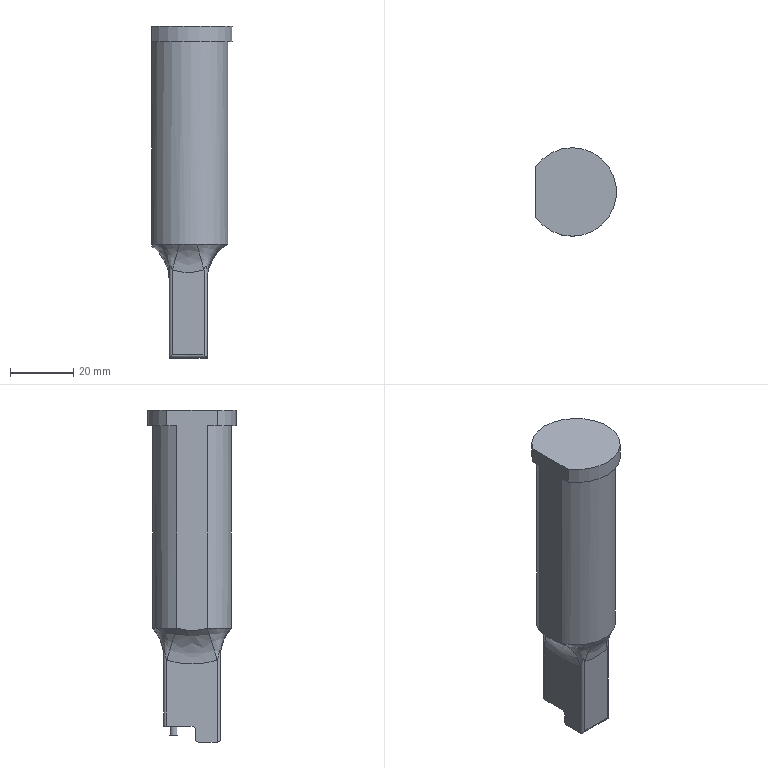Part | STEP file | lll_id3170_x_t | 1 solid | 29 faces | box 25.5 x 28 x 105 mm | volume 41911 mm3 | plane 11 | cylinder 10 | spline 8 | commonest cylinder face diameters 2 x7 2.4 x1 25 x1 28 x1
STEP:
#1=CARTESIAN_POINT('',(481.37,-342.601,87.5));
#2=VERTEX_POINT('',#1);
#3=CARTESIAN_POINT('',(481.37,-352.399,87.5));
#4=VERTEX_POINT('',#3);
#5=CARTESIAN_POINT('',(492.87,-347.5,87.5));
#6=DIRECTION('',(0.,0.,-1.));
#7=DIRECTION('',(-1.,0.,0.));
#8=AXIS2_PLACEMENT_3D('',#5,#6,#7);
#9=CIRCLE('',#8,12.5);
#10=EDGE_CURVE('',#2,#4,#9,.T.);
#11=ORIENTED_EDGE('',*,*,#10,.T.);
#12=CARTESIAN_POINT('',(481.37,-352.399,23.5));
#13=VERTEX_POINT('',#12);
#14=CARTESIAN_POINT('',(481.37,-352.399,-7.5));
#15=DIRECTION('',(0.,0.,1.));
#16=VECTOR('',#15,1.);
#17=LINE('',#14,#16);
#18=EDGE_CURVE('',#13,#4,#17,.T.);
#19=ORIENTED_EDGE('',*,*,#18,.F.);
#20=CARTESIAN_POINT('',(490.1,-359.689,23.5));
#21=VERTEX_POINT('',#20);
#22=CARTESIAN_POINT('',(490.1,-359.689,23.5));
#23=CARTESIAN_POINT('',(486.235,-358.811,23.5));
#24=CARTESIAN_POINT('',(482.924,-356.046,23.499));
#25=CARTESIAN_POINT('',(481.37,-352.399,23.5));
#26=B_SPLINE_CURVE_WITH_KNOTS('',3,(#22,#23,#24,#25),.UNSPECIFIED.,.F.,.F.,(4,4),(0.,1.),.UNSPECIFIED.);
#27=EDGE_CURVE('',#21,#13,#26,.T.);
#28=ORIENTED_EDGE('',*,*,#27,.F.);
#29=CARTESIAN_POINT('',(495.641,-359.689,23.5));
#30=VERTEX_POINT('',#29);
#31=CARTESIAN_POINT('',(495.641,-359.689,23.5));
#32=CARTESIAN_POINT('',(493.82,-360.103,23.5));
#33=CARTESIAN_POINT('',(491.921,-360.103,23.5));
#34=CARTESIAN_POINT('',(490.1,-359.689,23.5));
#35=B_SPLINE_CURVE_WITH_KNOTS('',3,(#31,#32,#33,#34),.UNSPECIFIED.,.F.,.F.,(4,4),(0.,1.),.UNSPECIFIED.);
#36=EDGE_CURVE('',#30,#21,#35,.T.);
#37=ORIENTED_EDGE('',*,*,#36,.F.);
#38=CARTESIAN_POINT('',(504.391,-352.351,23.5));
#39=VERTEX_POINT('',#38);
#40=CARTESIAN_POINT('',(504.391,-352.351,23.5));
#41=CARTESIAN_POINT('',(502.846,-356.02,23.5));
#42=CARTESIAN_POINT('',(499.523,-358.807,23.5));
#43=CARTESIAN_POINT('',(495.641,-359.689,23.5));
#44=B_SPLINE_CURVE_WITH_KNOTS('',3,(#40,#41,#42,#43),.UNSPECIFIED.,.F.,.F.,(4,4),(0.,1.),.UNSPECIFIED.);
#45=EDGE_CURVE('',#39,#30,#44,.T.);
#46=ORIENTED_EDGE('',*,*,#45,.F.);
#47=CARTESIAN_POINT('',(504.391,-342.649,23.5));
#48=VERTEX_POINT('',#47);
#49=CARTESIAN_POINT('',(504.391,-342.649,23.5));
#50=CARTESIAN_POINT('',(505.688,-345.731,23.5));
#51=CARTESIAN_POINT('',(505.688,-349.27,23.5));
#52=CARTESIAN_POINT('',(504.391,-352.351,23.5));
#53=B_SPLINE_CURVE_WITH_KNOTS('',3,(#49,#50,#51,#52),.UNSPECIFIED.,.F.,.F.,(4,4),(0.,1.),.UNSPECIFIED.);
#54=EDGE_CURVE('',#48,#39,#53,.T.);
#55=ORIENTED_EDGE('',*,*,#54,.F.);
#56=CARTESIAN_POINT('',(495.641,-335.311,23.5));
#57=VERTEX_POINT('',#56);
#58=CARTESIAN_POINT('',(495.641,-335.311,23.5));
#59=CARTESIAN_POINT('',(499.523,-336.193,23.5));
#60=CARTESIAN_POINT('',(502.846,-338.98,23.5));
#61=CARTESIAN_POINT('',(504.391,-342.649,23.5));
#62=B_SPLINE_CURVE_WITH_KNOTS('',3,(#58,#59,#60,#61),.UNSPECIFIED.,.F.,.F.,(4,4),(0.,1.),.UNSPECIFIED.);
#63=EDGE_CURVE('',#57,#48,#62,.T.);
#64=ORIENTED_EDGE('',*,*,#63,.F.);
#65=CARTESIAN_POINT('',(490.1,-335.311,23.5));
#66=VERTEX_POINT('',#65);
#67=CARTESIAN_POINT('',(490.1,-335.311,23.5));
#68=CARTESIAN_POINT('',(491.921,-334.897,23.5));
#69=CARTESIAN_POINT('',(493.82,-334.897,23.5));
#70=CARTESIAN_POINT('',(495.641,-335.311,23.5));
#71=B_SPLINE_CURVE_WITH_KNOTS('',3,(#67,#68,#69,#70),.UNSPECIFIED.,.F.,.F.,(4,4),(0.,1.),.UNSPECIFIED.);
#72=EDGE_CURVE('',#66,#57,#71,.T.);
#73=ORIENTED_EDGE('',*,*,#72,.F.);
#74=CARTESIAN_POINT('',(481.37,-342.601,23.5));
#75=VERTEX_POINT('',#74);
#76=CARTESIAN_POINT('',(481.37,-342.601,23.5));
#77=CARTESIAN_POINT('',(482.924,-338.955,23.5));
#78=CARTESIAN_POINT('',(486.235,-336.189,23.5));
#79=CARTESIAN_POINT('',(490.1,-335.311,23.5));
#80=B_SPLINE_CURVE_WITH_KNOTS('',3,(#76,#77,#78,#79),.UNSPECIFIED.,.F.,.F.,(4,4),(0.,1.),.UNSPECIFIED.);
#81=EDGE_CURVE('',#75,#66,#80,.T.);
#82=ORIENTED_EDGE('',*,*,#81,.F.);
#83=CARTESIAN_POINT('',(481.37,-342.601,-7.5));
#84=DIRECTION('',(0.,0.,-1.));
#85=VECTOR('',#84,1.);
#86=LINE('',#83,#85);
#87=EDGE_CURVE('',#2,#75,#86,.T.);
#88=ORIENTED_EDGE('',*,*,#87,.F.);
#89=EDGE_LOOP('',(#11,#19,#28,#37,#46,#55,#64,#73,#82,#88));
#90=FACE_OUTER_BOUND('',#89,.T.);
#91=CARTESIAN_POINT('',(492.87,-347.5,-7.5));
#92=DIRECTION('',(0.,0.,1.));
#93=DIRECTION('',(-1.,0.,0.));
#94=AXIS2_PLACEMENT_3D('',#91,#92,#93);
#95=CYLINDRICAL_SURFACE('',#94,12.5);
#96=ADVANCED_FACE('',(#90),#95,.T.);
#97=CARTESIAN_POINT('',(481.37,-355.484,87.5));
#98=VERTEX_POINT('',#97);
#99=CARTESIAN_POINT('',(481.37,-347.5,87.5));
#100=DIRECTION('',(0.,-1.,0.));
#101=VECTOR('',#100,1.);
#102=LINE('',#99,#101);
#103=EDGE_CURVE('',#4,#98,#102,.T.);
#104=ORIENTED_EDGE('',*,*,#103,.F.);
#105=ORIENTED_EDGE('',*,*,#10,.F.);
#106=CARTESIAN_POINT('',(481.37,-339.516,87.5));
#107=VERTEX_POINT('',#106);
#108=CARTESIAN_POINT('',(481.37,-347.5,87.5));
#109=DIRECTION('',(0.,-1.,0.));
#110=VECTOR('',#109,1.);
#111=LINE('',#108,#110);
#112=EDGE_CURVE('',#107,#2,#111,.T.);
#113=ORIENTED_EDGE('',*,*,#112,.F.);
#114=CARTESIAN_POINT('',(492.87,-347.5,87.5));
#115=DIRECTION('',(0.,0.,1.));
#116=DIRECTION('',(-1.,0.,0.));
#117=AXIS2_PLACEMENT_3D('',#114,#115,#116);
#118=CIRCLE('',#117,14.);
#119=EDGE_CURVE('',#98,#107,#118,.T.);
#120=ORIENTED_EDGE('',*,*,#119,.F.);
#121=EDGE_LOOP('',(#104,#105,#113,#120));
#122=FACE_OUTER_BOUND('',#121,.T.);
#123=CARTESIAN_POINT('',(492.87,-347.5,87.5));
#124=DIRECTION('',(0.,0.,1.));
#125=DIRECTION('',(-1.,0.,0.));
#126=AXIS2_PLACEMENT_3D('',#123,#124,#125);
#127=PLANE('',#126);
#128=ADVANCED_FACE('',(#122),#127,.F.);
#129=CARTESIAN_POINT('',(481.37,-355.484,92.5));
#130=VERTEX_POINT('',#129);
#131=CARTESIAN_POINT('',(481.37,-339.516,92.5));
#132=VERTEX_POINT('',#131);
#133=CARTESIAN_POINT('',(492.87,-347.5,92.5));
#134=DIRECTION('',(0.,0.,1.));
#135=DIRECTION('',(1.,0.,0.));
#136=AXIS2_PLACEMENT_3D('',#133,#134,#135);
#137=CIRCLE('',#136,14.);
#138=EDGE_CURVE('',#130,#132,#137,.T.);
#139=ORIENTED_EDGE('',*,*,#138,.T.);
#140=CARTESIAN_POINT('',(481.37,-21.,92.5));
#141=DIRECTION('',(0.,1.,0.));
#142=VECTOR('',#141,1.);
#143=LINE('',#140,#142);
#144=EDGE_CURVE('',#130,#132,#143,.T.);
#145=ORIENTED_EDGE('',*,*,#144,.F.);
#146=EDGE_LOOP('',(#139,#145));
#147=FACE_OUTER_BOUND('',#146,.T.);
#148=CARTESIAN_POINT('',(444.,-21.,92.5));
#149=DIRECTION('',(0.,0.,-1.));
#150=DIRECTION('',(1.,0.,0.));
#151=AXIS2_PLACEMENT_3D('',#148,#149,#150);
#152=PLANE('',#151);
#153=ADVANCED_FACE('',(#147),#152,.F.);
#154=ORIENTED_EDGE('',*,*,#138,.F.);
#155=CARTESIAN_POINT('',(481.37,-355.484,-7.5));
#156=DIRECTION('',(0.,0.,1.));
#157=VECTOR('',#156,1.);
#158=LINE('',#155,#157);
#159=EDGE_CURVE('',#98,#130,#158,.T.);
#160=ORIENTED_EDGE('',*,*,#159,.F.);
#161=ORIENTED_EDGE('',*,*,#119,.T.);
#162=CARTESIAN_POINT('',(481.37,-339.516,-7.5));
#163=DIRECTION('',(0.,0.,-1.));
#164=VECTOR('',#163,1.);
#165=LINE('',#162,#164);
#166=EDGE_CURVE('',#132,#107,#165,.T.);
#167=ORIENTED_EDGE('',*,*,#166,.F.);
#168=EDGE_LOOP('',(#154,#160,#161,#167));
#169=FACE_OUTER_BOUND('',#168,.T.);
#170=CARTESIAN_POINT('',(492.87,-347.5,-7.5));
#171=DIRECTION('',(0.,0.,1.));
#172=DIRECTION('',(-1.,0.,0.));
#173=AXIS2_PLACEMENT_3D('',#170,#171,#172);
#174=CYLINDRICAL_SURFACE('',#173,14.);
#175=ADVANCED_FACE('',(#169),#174,.T.);
#176=CARTESIAN_POINT('',(481.37,-352.355,23.486));
#177=VERTEX_POINT('',#176);
#178=CARTESIAN_POINT('',(481.37,-352.399,23.5));
#179=CARTESIAN_POINT('',(481.37,-352.384,23.495));
#180=CARTESIAN_POINT('',(481.37,-352.37,23.491));
#181=CARTESIAN_POINT('',(481.37,-352.355,23.486));
#182=B_SPLINE_CURVE_WITH_KNOTS('',3,(#178,#179,#180,#181),.UNSPECIFIED.,.F.,.F.,(4,4),(0.,1.),.UNSPECIFIED.);
#183=EDGE_CURVE('',#13,#177,#182,.T.);
#184=ORIENTED_EDGE('',*,*,#183,.T.);
#185=CARTESIAN_POINT('',(486.87,-355.5,13.344));
#186=VERTEX_POINT('',#185);
#187=CARTESIAN_POINT('',(473.87,-355.5,13.344));
#188=DIRECTION('',(0.,0.9551,-0.2962));
#189=DIRECTION('',(0.,-0.2962,-0.9551));
#190=AXIS2_PLACEMENT_3D('',#187,#188,#189);
#191=CIRCLE('',#190,13.);
#192=EDGE_CURVE('',#177,#186,#191,.T.);
#193=ORIENTED_EDGE('',*,*,#192,.T.);
#194=CARTESIAN_POINT('',(487.87,-356.5,15.267));
#195=VERTEX_POINT('',#194);
#196=CARTESIAN_POINT('',(486.87,-355.5,13.344));
#197=CARTESIAN_POINT('',(486.87,-355.629,13.906));
#198=CARTESIAN_POINT('',(486.895,-355.755,14.475));
#199=CARTESIAN_POINT('',(486.992,-355.995,15.517));
#200=CARTESIAN_POINT('',(487.065,-356.107,15.974));
#201=CARTESIAN_POINT('',(487.251,-356.296,16.492));
#202=CARTESIAN_POINT('',(487.365,-356.373,16.537));
#203=CARTESIAN_POINT('',(487.61,-356.475,16.162));
#204=CARTESIAN_POINT('',(487.743,-356.5,15.752));
#205=CARTESIAN_POINT('',(487.87,-356.5,15.267));
#206=(BOUNDED_CURVE()B_SPLINE_CURVE(3,(#196,#197,#198,#199,#200,#201,#202,#203,#204,#205),.UNSPECIFIED.,.F.,.F.)B_SPLINE_CURVE_WITH_KNOTS((4,2,2,2,4),(0.,0.25,0.5,0.75,1.),.UNSPECIFIED.)CURVE()GEOMETRIC_REPRESENTATION_ITEM()RATIONAL_B_SPLINE_CURVE((1.,1.,1.,1.,1.,1.,1.,1.,1.,1.))REPRESENTATION_ITEM(''));
#207=EDGE_CURVE('',#186,#195,#206,.T.);
#208=ORIENTED_EDGE('',*,*,#207,.T.);
#209=CARTESIAN_POINT('',(487.87,-369.5,15.267));
#210=DIRECTION('',(0.9652,0.,-0.2614));
#211=DIRECTION('',(0.2614,0.,0.9652));
#212=AXIS2_PLACEMENT_3D('',#209,#210,#211);
#213=CIRCLE('',#212,13.);
#214=EDGE_CURVE('',#195,#21,#213,.T.);
#215=ORIENTED_EDGE('',*,*,#214,.T.);
#216=ORIENTED_EDGE('',*,*,#27,.T.);
#217=EDGE_LOOP('',(#184,#193,#208,#215,#216));
#218=FACE_OUTER_BOUND('',#217,.T.);
#219=CARTESIAN_POINT('',(486.87,-355.5,13.344));
#220=CARTESIAN_POINT('',(486.87,-353.501,19.791));
#221=CARTESIAN_POINT('',(481.35,-352.351,23.5));
#222=CARTESIAN_POINT('',(486.87,-355.629,13.906));
#223=CARTESIAN_POINT('',(486.616,-353.761,19.745));
#224=CARTESIAN_POINT('',(481.743,-353.285,23.5));
#225=CARTESIAN_POINT('',(486.895,-355.755,14.475));
#226=CARTESIAN_POINT('',(486.443,-354.143,19.805));
#227=CARTESIAN_POINT('',(482.223,-354.123,23.5));
#228=CARTESIAN_POINT('',(486.992,-355.995,15.517));
#229=CARTESIAN_POINT('',(486.389,-354.985,20.001));
#230=CARTESIAN_POINT('',(483.391,-355.708,23.5));
#231=CARTESIAN_POINT('',(487.065,-356.107,15.974));
#232=CARTESIAN_POINT('',(486.509,-355.437,20.135));
#233=CARTESIAN_POINT('',(484.07,-356.432,23.5));
#234=CARTESIAN_POINT('',(487.251,-356.296,16.492));
#235=CARTESIAN_POINT('',(487.023,-356.169,20.292));
#236=CARTESIAN_POINT('',(485.587,-357.707,23.5));
#237=CARTESIAN_POINT('',(487.365,-356.373,16.537));
#238=CARTESIAN_POINT('',(487.422,-356.453,20.308));
#239=CARTESIAN_POINT('',(486.438,-358.263,23.5));
#240=CARTESIAN_POINT('',(487.61,-356.475,16.162));
#241=CARTESIAN_POINT('',(488.285,-356.698,20.191));
#242=CARTESIAN_POINT('',(488.213,-359.142,23.5));
#243=CARTESIAN_POINT('',(487.743,-356.5,15.752));
#244=CARTESIAN_POINT('',(488.759,-356.66,20.063));
#245=CARTESIAN_POINT('',(489.162,-359.476,23.5));
#246=CARTESIAN_POINT('',(487.87,-356.5,15.267));
#247=CARTESIAN_POINT('',(489.141,-356.5,19.959));
#248=CARTESIAN_POINT('',(490.1,-359.689,23.5));
#249=(BOUNDED_SURFACE()B_SPLINE_SURFACE(3,2,((#219,#220,#221),(#222,#223,#224),(#225,#226,#227),(#228,#229,#230),(#231,#232,#233),(#234,#235,#236),(#237,#238,#239),(#240,#241,#242),(#243,#244,#245),(#246,#247,#248)),.UNSPECIFIED.,.F.,.F.,.F.)B_SPLINE_SURFACE_WITH_KNOTS((4,2,2,2,4),(3,3),(0.,0.25,0.5,0.75,1.),(0.,1.),.UNSPECIFIED.)GEOMETRIC_REPRESENTATION_ITEM()RATIONAL_B_SPLINE_SURFACE(((1.,0.8875,1.),(1.,0.9048,1.),(1.,0.9192,1.),(1.,0.9424,1.),(1.,0.9508,1.),(1.,0.96,1.),(1.,0.9607,1.),(1.,0.9542,1.),(1.,0.9469,1.),(1.,0.9367,1.)))REPRESENTATION_ITEM('')SURFACE());
#250=ADVANCED_FACE('',(#218),#249,.T.);
#251=CARTESIAN_POINT('',(481.37,-342.645,23.486));
#252=VERTEX_POINT('',#251);
#253=CARTESIAN_POINT('',(481.37,-352.355,23.486));
#254=CARTESIAN_POINT('',(481.37,-350.783,22.999));
#255=CARTESIAN_POINT('',(481.37,-349.135,22.86));
#256=CARTESIAN_POINT('',(481.37,-345.863,22.86));
#257=CARTESIAN_POINT('',(481.37,-344.22,22.998));
#258=CARTESIAN_POINT('',(481.37,-342.645,23.486));
#259=B_SPLINE_CURVE_WITH_KNOTS('',3,(#253,#254,#255,#256,#257,#258),.UNSPECIFIED.,.F.,.F.,(4,2,4),(0.,0.5,1.),.UNSPECIFIED.);
#260=EDGE_CURVE('',#177,#252,#259,.T.);
#261=ORIENTED_EDGE('',*,*,#260,.T.);
#262=CARTESIAN_POINT('',(486.87,-339.5,13.344));
#263=VERTEX_POINT('',#262);
#264=CARTESIAN_POINT('',(473.87,-339.5,13.344));
#265=DIRECTION('',(0.,0.9551,0.2962));
#266=DIRECTION('',(0.,0.2962,-0.9551));
#267=AXIS2_PLACEMENT_3D('',#264,#265,#266);
#268=CIRCLE('',#267,13.);
#269=EDGE_CURVE('',#252,#263,#268,.T.);
#270=ORIENTED_EDGE('',*,*,#269,.T.);
#271=CARTESIAN_POINT('',(486.87,-339.5,13.344));
#272=CARTESIAN_POINT('',(486.87,-342.08,12.544));
#273=CARTESIAN_POINT('',(486.87,-344.771,12.243));
#274=CARTESIAN_POINT('',(486.87,-350.203,12.241));
#275=CARTESIAN_POINT('',(486.87,-352.893,12.536));
#276=CARTESIAN_POINT('',(486.87,-355.5,13.344));
#277=B_SPLINE_CURVE_WITH_KNOTS('',3,(#271,#272,#273,#274,#275,#276),.UNSPECIFIED.,.F.,.F.,(4,2,4),(0.,0.5,1.),.UNSPECIFIED.);
#278=EDGE_CURVE('',#263,#186,#277,.T.);
#279=ORIENTED_EDGE('',*,*,#278,.T.);
#280=ORIENTED_EDGE('',*,*,#192,.F.);
#281=EDGE_LOOP('',(#261,#270,#279,#280));
#282=FACE_OUTER_BOUND('',#281,.T.);
#283=CARTESIAN_POINT('',(486.87,-339.5,13.344));
#284=CARTESIAN_POINT('',(486.87,-341.499,19.791));
#285=CARTESIAN_POINT('',(481.35,-342.649,23.5));
#286=CARTESIAN_POINT('',(486.87,-342.068,12.548));
#287=CARTESIAN_POINT('',(486.87,-343.348,19.674));
#288=CARTESIAN_POINT('',(480.798,-343.961,23.5));
#289=CARTESIAN_POINT('',(486.87,-344.771,12.243));
#290=CARTESIAN_POINT('',(486.87,-345.394,19.747));
#291=CARTESIAN_POINT('',(480.372,-345.705,23.5));
#292=CARTESIAN_POINT('',(486.87,-350.203,12.241));
#293=CARTESIAN_POINT('',(486.87,-349.586,19.747));
#294=CARTESIAN_POINT('',(480.369,-349.278,23.5));
#295=CARTESIAN_POINT('',(486.87,-352.886,12.534));
#296=CARTESIAN_POINT('',(486.87,-351.616,19.672));
#297=CARTESIAN_POINT('',(480.787,-351.013,23.5));
#298=CARTESIAN_POINT('',(486.87,-355.5,13.344));
#299=CARTESIAN_POINT('',(486.87,-353.501,19.791));
#300=CARTESIAN_POINT('',(481.35,-352.351,23.5));
#301=(BOUNDED_SURFACE()B_SPLINE_SURFACE(3,2,((#283,#284,#285),(#286,#287,#288),(#289,#290,#291),(#292,#293,#294),(#295,#296,#297),(#298,#299,#300)),.UNSPECIFIED.,.F.,.F.,.F.)B_SPLINE_SURFACE_WITH_KNOTS((4,2,4),(3,3),(0.,0.5,1.),(0.,1.),.UNSPECIFIED.)GEOMETRIC_REPRESENTATION_ITEM()RATIONAL_B_SPLINE_SURFACE(((1.,0.8875,1.),(1.,0.8752,1.),(1.,0.8661,1.),(1.,0.866,1.),(1.,0.875,1.),(1.,0.8875,1.)))REPRESENTATION_ITEM('')SURFACE());
#302=ADVANCED_FACE('',(#282),#301,.T.);
#303=CARTESIAN_POINT('',(481.37,-342.601,23.5));
#304=CARTESIAN_POINT('',(481.37,-342.616,23.495));
#305=CARTESIAN_POINT('',(481.37,-342.63,23.491));
#306=CARTESIAN_POINT('',(481.37,-342.645,23.486));
#307=B_SPLINE_CURVE_WITH_KNOTS('',3,(#303,#304,#305,#306),.UNSPECIFIED.,.F.,.F.,(4,4),(0.,1.),.UNSPECIFIED.);
#308=EDGE_CURVE('',#75,#252,#307,.T.);
#309=ORIENTED_EDGE('',*,*,#308,.F.);
#310=ORIENTED_EDGE('',*,*,#81,.T.);
#311=CARTESIAN_POINT('',(487.87,-338.5,15.267));
#312=VERTEX_POINT('',#311);
#313=CARTESIAN_POINT('',(487.87,-325.5,15.267));
#314=DIRECTION('',(0.9652,0.,-0.2614));
#315=DIRECTION('',(-0.2614,0.,-0.9652));
#316=AXIS2_PLACEMENT_3D('',#313,#314,#315);
#317=CIRCLE('',#316,13.);
#318=EDGE_CURVE('',#66,#312,#317,.T.);
#319=ORIENTED_EDGE('',*,*,#318,.T.);
#320=CARTESIAN_POINT('',(487.87,-338.5,15.267));
#321=CARTESIAN_POINT('',(487.741,-338.5,15.757));
#322=CARTESIAN_POINT('',(487.609,-338.526,16.165));
#323=CARTESIAN_POINT('',(487.425,-338.602,16.444));
#324=CARTESIAN_POINT('',(487.365,-338.635,16.484));
#325=CARTESIAN_POINT('',(487.254,-338.71,16.441));
#326=CARTESIAN_POINT('',(487.203,-338.752,16.361));
#327=CARTESIAN_POINT('',(487.064,-338.894,15.97));
#328=CARTESIAN_POINT('',(486.992,-339.005,15.517));
#329=CARTESIAN_POINT('',(486.895,-339.246,14.474));
#330=CARTESIAN_POINT('',(486.87,-339.372,13.9));
#331=CARTESIAN_POINT('',(486.87,-339.5,13.344));
#332=(BOUNDED_CURVE()B_SPLINE_CURVE(3,(#320,#321,#322,#323,#324,#325,#326,#327,#328,#329,#330,#331),.UNSPECIFIED.,.F.,.F.)B_SPLINE_CURVE_WITH_KNOTS((4,2,2,2,2,4),(0.,0.25,0.375,0.5,0.75,1.),.UNSPECIFIED.)CURVE()GEOMETRIC_REPRESENTATION_ITEM()RATIONAL_B_SPLINE_CURVE((1.,1.,1.,1.,1.,1.,1.,1.,1.,1.,1.,1.))REPRESENTATION_ITEM(''));
#333=EDGE_CURVE('',#312,#263,#332,.T.);
#334=ORIENTED_EDGE('',*,*,#333,.T.);
#335=ORIENTED_EDGE('',*,*,#269,.F.);
#336=EDGE_LOOP('',(#309,#310,#319,#334,#335));
#337=FACE_OUTER_BOUND('',#336,.T.);
#338=CARTESIAN_POINT('',(487.87,-338.5,15.267));
#339=CARTESIAN_POINT('',(489.141,-338.5,19.959));
#340=CARTESIAN_POINT('',(490.1,-335.311,23.5));
#341=CARTESIAN_POINT('',(487.741,-338.5,15.757));
#342=CARTESIAN_POINT('',(488.754,-338.338,20.065));
#343=CARTESIAN_POINT('',(489.151,-335.527,23.5));
#344=CARTESIAN_POINT('',(487.609,-338.526,16.165));
#345=CARTESIAN_POINT('',(488.281,-338.303,20.192));
#346=CARTESIAN_POINT('',(488.206,-335.86,23.5));
#347=CARTESIAN_POINT('',(487.425,-338.602,16.444));
#348=CARTESIAN_POINT('',(487.632,-338.488,20.28));
#349=CARTESIAN_POINT('',(486.872,-336.522,23.5));
#350=CARTESIAN_POINT('',(487.365,-338.635,16.484));
#351=CARTESIAN_POINT('',(487.421,-338.589,20.293));
#352=CARTESIAN_POINT('',(486.432,-336.774,23.5));
#353=CARTESIAN_POINT('',(487.254,-338.71,16.441));
#354=CARTESIAN_POINT('',(487.052,-338.853,20.279));
#355=CARTESIAN_POINT('',(485.597,-337.322,23.5));
#356=CARTESIAN_POINT('',(487.203,-338.752,16.361));
#357=CARTESIAN_POINT('',(486.893,-339.015,20.253));
#358=CARTESIAN_POINT('',(485.201,-337.617,23.5));
#359=CARTESIAN_POINT('',(487.064,-338.894,15.97));
#360=CARTESIAN_POINT('',(486.507,-339.567,20.133));
#361=CARTESIAN_POINT('',(484.062,-338.575,23.5));
#362=CARTESIAN_POINT('',(486.992,-339.005,15.517));
#363=CARTESIAN_POINT('',(486.389,-340.015,20.001));
#364=CARTESIAN_POINT('',(483.391,-339.292,23.5));
#365=CARTESIAN_POINT('',(486.895,-339.246,14.474));
#366=CARTESIAN_POINT('',(486.443,-340.858,19.804));
#367=CARTESIAN_POINT('',(482.223,-340.879,23.5));
#368=CARTESIAN_POINT('',(486.87,-339.372,13.9));
#369=CARTESIAN_POINT('',(486.618,-341.241,19.745));
#370=CARTESIAN_POINT('',(481.74,-341.724,23.5));
#371=CARTESIAN_POINT('',(486.87,-339.5,13.344));
#372=CARTESIAN_POINT('',(486.87,-341.499,19.791));
#373=CARTESIAN_POINT('',(481.35,-342.649,23.5));
#374=(BOUNDED_SURFACE()B_SPLINE_SURFACE(3,2,((#338,#339,#340),(#341,#342,#343),(#344,#345,#346),(#347,#348,#349),(#350,#351,#352),(#353,#354,#355),(#356,#357,#358),(#359,#360,#361),(#362,#363,#364),(#365,#366,#367),(#368,#369,#370),(#371,#372,#373)),.UNSPECIFIED.,.F.,.F.,.F.)B_SPLINE_SURFACE_WITH_KNOTS((4,2,2,2,2,4),(3,3),(0.,0.25,0.375,0.5,0.75,1.),(0.,1.),.UNSPECIFIED.)GEOMETRIC_REPRESENTATION_ITEM()RATIONAL_B_SPLINE_SURFACE(((1.,0.9367,1.),(1.,0.947,1.),(1.,0.9542,1.),(1.,0.9591,1.),(1.,0.9597,1.),(1.,0.959,1.),(1.,0.9576,1.),(1.,0.9507,1.),(1.,0.9424,1.),(1.,0.9192,1.),(1.,0.9047,1.),(1.,0.8875,1.)))REPRESENTATION_ITEM('')SURFACE());
#375=ADVANCED_FACE('',(#337),#374,.T.);
#376=CARTESIAN_POINT('',(491.67,-341.7,-7.5));
#377=VERTEX_POINT('',#376);
#378=CARTESIAN_POINT('',(492.87,-341.7,-7.5));
#379=DIRECTION('',(0.,0.,1.));
#380=DIRECTION('',(-1.,0.,0.));
#381=AXIS2_PLACEMENT_3D('',#378,#379,#380);
#382=CIRCLE('',#381,1.2);
#383=EDGE_CURVE('',#377,#377,#382,.T.);
#384=ORIENTED_EDGE('',*,*,#383,.T.);
#385=EDGE_LOOP('',(#384));
#386=FACE_BOUND('',#385,.T.);
#387=CARTESIAN_POINT('',(486.87,-339.5,-7.5));
#388=VERTEX_POINT('',#387);
#389=CARTESIAN_POINT('',(486.87,-347.5,-7.5));
#390=VERTEX_POINT('',#389);
#391=CARTESIAN_POINT('',(486.87,-339.5,-7.5));
#392=DIRECTION('',(0.,-1.,0.));
#393=VECTOR('',#392,1.);
#394=LINE('',#391,#393);
#395=EDGE_CURVE('',#388,#390,#394,.T.);
#396=ORIENTED_EDGE('',*,*,#395,.F.);
#397=CARTESIAN_POINT('',(487.87,-338.5,-7.5));
#398=VERTEX_POINT('',#397);
#399=CARTESIAN_POINT('',(487.87,-339.5,-7.5));
#400=DIRECTION('',(0.,0.,1.));
#401=DIRECTION('',(-1.,0.,0.));
#402=AXIS2_PLACEMENT_3D('',#399,#400,#401);
#403=CIRCLE('',#402,1.);
#404=EDGE_CURVE('',#398,#388,#403,.T.);
#405=ORIENTED_EDGE('',*,*,#404,.F.);
#406=CARTESIAN_POINT('',(497.87,-338.5,-7.5));
#407=VERTEX_POINT('',#406);
#408=CARTESIAN_POINT('',(497.87,-338.5,-7.5));
#409=DIRECTION('',(-1.,0.,0.));
#410=VECTOR('',#409,1.);
#411=LINE('',#408,#410);
#412=EDGE_CURVE('',#407,#398,#411,.T.);
#413=ORIENTED_EDGE('',*,*,#412,.F.);
#414=CARTESIAN_POINT('',(498.87,-339.5,-7.5));
#415=VERTEX_POINT('',#414);
#416=CARTESIAN_POINT('',(497.87,-339.5,-7.5));
#417=DIRECTION('',(0.,0.,1.));
#418=DIRECTION('',(-1.,0.,0.));
#419=AXIS2_PLACEMENT_3D('',#416,#417,#418);
#420=CIRCLE('',#419,1.);
#421=EDGE_CURVE('',#415,#407,#420,.T.);
#422=ORIENTED_EDGE('',*,*,#421,.F.);
#423=CARTESIAN_POINT('',(498.87,-347.5,-7.5));
#424=VERTEX_POINT('',#423);
#425=CARTESIAN_POINT('',(498.87,-355.5,-7.5));
#426=DIRECTION('',(0.,1.,0.));
#427=VECTOR('',#426,1.);
#428=LINE('',#425,#427);
#429=EDGE_CURVE('',#424,#415,#428,.T.);
#430=ORIENTED_EDGE('',*,*,#429,.F.);
#431=CARTESIAN_POINT('',(497.87,-347.5,-7.5));
#432=DIRECTION('',(1.,0.,0.));
#433=VECTOR('',#432,1.);
#434=LINE('',#431,#433);
#435=EDGE_CURVE('',#390,#424,#434,.T.);
#436=ORIENTED_EDGE('',*,*,#435,.F.);
#437=EDGE_LOOP('',(#396,#405,#413,#422,#430,#436));
#438=FACE_BOUND('',#437,.T.);
#439=CARTESIAN_POINT('',(497.87,-339.5,-7.5));
#440=DIRECTION('',(0.,0.,-1.));
#441=DIRECTION('',(-1.,0.,0.));
#442=AXIS2_PLACEMENT_3D('',#439,#440,#441);
#443=PLANE('',#442);
#444=ADVANCED_FACE('',(#386,#438),#443,.T.);
#445=CARTESIAN_POINT('',(497.87,-356.5,-11.5));
#446=VERTEX_POINT('',#445);
#447=CARTESIAN_POINT('',(497.87,-356.5,15.267));
#448=VERTEX_POINT('',#447);
#449=CARTESIAN_POINT('',(497.87,-356.5,-7.5));
#450=DIRECTION('',(0.,0.,1.));
#451=VECTOR('',#450,1.);
#452=LINE('',#449,#451);
#453=EDGE_CURVE('',#446,#448,#452,.T.);
#454=ORIENTED_EDGE('',*,*,#453,.T.);
#455=CARTESIAN_POINT('',(487.87,-356.5,15.267));
#456=CARTESIAN_POINT('',(489.495,-356.5,14.827));
#457=CARTESIAN_POINT('',(491.197,-356.5,14.626));
#458=CARTESIAN_POINT('',(494.549,-356.5,14.626));
#459=CARTESIAN_POINT('',(496.228,-356.5,14.823));
#460=CARTESIAN_POINT('',(497.87,-356.5,15.267));
#461=B_SPLINE_CURVE_WITH_KNOTS('',3,(#455,#456,#457,#458,#459,#460),.UNSPECIFIED.,.F.,.F.,(4,2,4),(0.,0.5,1.),.UNSPECIFIED.);
#462=EDGE_CURVE('',#195,#448,#461,.T.);
#463=ORIENTED_EDGE('',*,*,#462,.F.);
#464=CARTESIAN_POINT('',(487.87,-356.5,-11.5));
#465=VERTEX_POINT('',#464);
#466=CARTESIAN_POINT('',(487.87,-356.5,-7.5));
#467=DIRECTION('',(0.,0.,1.));
#468=VECTOR('',#467,1.);
#469=LINE('',#466,#468);
#470=EDGE_CURVE('',#465,#195,#469,.T.);
#471=ORIENTED_EDGE('',*,*,#470,.F.);
#472=CARTESIAN_POINT('',(487.87,-356.5,-11.5));
#473=DIRECTION('',(-1.,0.,0.));
#474=VECTOR('',#473,1.);
#475=LINE('',#472,#474);
#476=EDGE_CURVE('',#446,#465,#475,.T.);
#477=ORIENTED_EDGE('',*,*,#476,.F.);
#478=EDGE_LOOP('',(#454,#463,#471,#477));
#479=FACE_OUTER_BOUND('',#478,.T.);
#480=CARTESIAN_POINT('',(487.87,-356.5,-7.5));
#481=DIRECTION('',(0.,-1.,0.));
#482=DIRECTION('',(1.,0.,0.));
#483=AXIS2_PLACEMENT_3D('',#480,#481,#482);
#484=PLANE('',#483);
#485=ADVANCED_FACE('',(#479),#484,.T.);
#486=ORIENTED_EDGE('',*,*,#470,.T.);
#487=ORIENTED_EDGE('',*,*,#207,.F.);
#488=CARTESIAN_POINT('',(486.87,-355.5,-12.5));
#489=VERTEX_POINT('',#488);
#490=CARTESIAN_POINT('',(486.87,-355.5,-7.5));
#491=DIRECTION('',(0.,0.,1.));
#492=VECTOR('',#491,1.);
#493=LINE('',#490,#492);
#494=EDGE_CURVE('',#489,#186,#493,.T.);
#495=ORIENTED_EDGE('',*,*,#494,.F.);
#496=CARTESIAN_POINT('',(487.87,-355.5,-11.5));
#497=DIRECTION('',(0.7071,0.,-0.7071));
#498=DIRECTION('',(-0.7071,0.,-0.7071));
#499=AXIS2_PLACEMENT_3D('',#496,#497,#498);
#500=ELLIPSE('',#499,1.414,1.);
#501=EDGE_CURVE('',#465,#489,#500,.T.);
#502=ORIENTED_EDGE('',*,*,#501,.F.);
#503=EDGE_LOOP('',(#486,#487,#495,#502));
#504=FACE_OUTER_BOUND('',#503,.T.);
#505=CARTESIAN_POINT('',(487.87,-355.5,-7.5));
#506=DIRECTION('',(0.,0.,-1.));
#507=DIRECTION('',(1.,0.,0.));
#508=AXIS2_PLACEMENT_3D('',#505,#506,#507);
#509=CYLINDRICAL_SURFACE('',#508,1.);
#510=ADVANCED_FACE('',(#504),#509,.T.);
#511=CARTESIAN_POINT('',(486.87,-349.5,-12.5));
#512=VERTEX_POINT('',#511);
#513=CARTESIAN_POINT('',(486.87,-339.5,-12.5));
#514=DIRECTION('',(0.,-1.,0.));
#515=VECTOR('',#514,1.);
#516=LINE('',#513,#515);
#517=EDGE_CURVE('',#512,#489,#516,.T.);
#518=ORIENTED_EDGE('',*,*,#517,.T.);
#519=ORIENTED_EDGE('',*,*,#494,.T.);
#520=ORIENTED_EDGE('',*,*,#278,.F.);
#521=CARTESIAN_POINT('',(486.87,-339.5,-7.5));
#522=DIRECTION('',(0.,0.,1.));
#523=VECTOR('',#522,1.);
#524=LINE('',#521,#523);
#525=EDGE_CURVE('',#388,#263,#524,.T.);
#526=ORIENTED_EDGE('',*,*,#525,.F.);
#527=ORIENTED_EDGE('',*,*,#395,.T.);
#528=CARTESIAN_POINT('',(486.87,-348.5,-8.5));
#529=VERTEX_POINT('',#528);
#530=CARTESIAN_POINT('',(486.87,-347.5,-8.5));
#531=DIRECTION('',(-1.,0.,0.));
#532=DIRECTION('',(0.,0.,-1.));
#533=AXIS2_PLACEMENT_3D('',#530,#531,#532);
#534=CIRCLE('',#533,1.);
#535=EDGE_CURVE('',#529,#390,#534,.T.);
#536=ORIENTED_EDGE('',*,*,#535,.F.);
#537=CARTESIAN_POINT('',(486.87,-348.5,-11.5));
#538=VERTEX_POINT('',#537);
#539=CARTESIAN_POINT('',(486.87,-348.5,-7.5));
#540=DIRECTION('',(0.,0.,1.));
#541=VECTOR('',#540,1.);
#542=LINE('',#539,#541);
#543=EDGE_CURVE('',#538,#529,#542,.T.);
#544=ORIENTED_EDGE('',*,*,#543,.F.);
#545=CARTESIAN_POINT('',(486.87,-349.5,-11.5));
#546=DIRECTION('',(1.,0.,0.));
#547=DIRECTION('',(0.,0.,-1.));
#548=AXIS2_PLACEMENT_3D('',#545,#546,#547);
#549=CIRCLE('',#548,1.);
#550=EDGE_CURVE('',#512,#538,#549,.T.);
#551=ORIENTED_EDGE('',*,*,#550,.F.);
#552=EDGE_LOOP('',(#518,#519,#520,#526,#527,#536,#544,#551));
#553=FACE_OUTER_BOUND('',#552,.T.);
#554=CARTESIAN_POINT('',(486.87,-339.5,-7.5));
#555=DIRECTION('',(-1.,0.,0.));
#556=DIRECTION('',(0.,-1.,0.));
#557=AXIS2_PLACEMENT_3D('',#554,#555,#556);
#558=PLANE('',#557);
#559=ADVANCED_FACE('',(#553),#558,.T.);
#560=CARTESIAN_POINT('',(487.87,-338.5,-7.5));
#561=DIRECTION('',(0.,0.,1.));
#562=VECTOR('',#561,1.);
#563=LINE('',#560,#562);
#564=EDGE_CURVE('',#398,#312,#563,.T.);
#565=ORIENTED_EDGE('',*,*,#564,.F.);
#566=ORIENTED_EDGE('',*,*,#404,.T.);
#567=ORIENTED_EDGE('',*,*,#525,.T.);
#568=ORIENTED_EDGE('',*,*,#333,.F.);
#569=EDGE_LOOP('',(#565,#566,#567,#568));
#570=FACE_OUTER_BOUND('',#569,.T.);
#571=CARTESIAN_POINT('',(487.87,-339.5,-7.5));
#572=DIRECTION('',(0.,0.,-1.));
#573=DIRECTION('',(1.,0.,0.));
#574=AXIS2_PLACEMENT_3D('',#571,#572,#573);
#575=CYLINDRICAL_SURFACE('',#574,1.);
#576=ADVANCED_FACE('',(#570),#575,.T.);
#577=CARTESIAN_POINT('',(497.87,-338.5,15.267));
#578=VERTEX_POINT('',#577);
#579=CARTESIAN_POINT('',(497.87,-338.5,-7.5));
#580=DIRECTION('',(0.,0.,1.));
#581=VECTOR('',#580,1.);
#582=LINE('',#579,#581);
#583=EDGE_CURVE('',#407,#578,#582,.T.);
#584=ORIENTED_EDGE('',*,*,#583,.F.);
#585=ORIENTED_EDGE('',*,*,#412,.T.);
#586=ORIENTED_EDGE('',*,*,#564,.T.);
#587=CARTESIAN_POINT('',(497.87,-338.5,15.267));
#588=CARTESIAN_POINT('',(496.246,-338.5,14.827));
#589=CARTESIAN_POINT('',(494.544,-338.5,14.626));
#590=CARTESIAN_POINT('',(491.192,-338.5,14.626));
#591=CARTESIAN_POINT('',(489.513,-338.5,14.823));
#592=CARTESIAN_POINT('',(487.87,-338.5,15.267));
#593=B_SPLINE_CURVE_WITH_KNOTS('',3,(#587,#588,#589,#590,#591,#592),.UNSPECIFIED.,.F.,.F.,(4,2,4),(0.,0.5,1.),.UNSPECIFIED.);
#594=EDGE_CURVE('',#578,#312,#593,.T.);
#595=ORIENTED_EDGE('',*,*,#594,.F.);
#596=EDGE_LOOP('',(#584,#585,#586,#595));
#597=FACE_OUTER_BOUND('',#596,.T.);
#598=CARTESIAN_POINT('',(497.87,-338.5,-7.5));
#599=DIRECTION('',(0.,1.,0.));
#600=DIRECTION('',(-1.,0.,0.));
#601=AXIS2_PLACEMENT_3D('',#598,#599,#600);
#602=PLANE('',#601);
#603=ADVANCED_FACE('',(#597),#602,.T.);
#604=CARTESIAN_POINT('',(498.87,-339.5,13.344));
#605=VERTEX_POINT('',#604);
#606=CARTESIAN_POINT('',(498.87,-339.5,-7.5));
#607=DIRECTION('',(0.,0.,1.));
#608=VECTOR('',#607,1.);
#609=LINE('',#606,#608);
#610=EDGE_CURVE('',#415,#605,#609,.T.);
#611=ORIENTED_EDGE('',*,*,#610,.F.);
#612=ORIENTED_EDGE('',*,*,#421,.T.);
#613=ORIENTED_EDGE('',*,*,#583,.T.);
#614=CARTESIAN_POINT('',(498.87,-339.5,13.344));
#615=CARTESIAN_POINT('',(498.87,-339.371,13.906));
#616=CARTESIAN_POINT('',(498.846,-339.245,14.475));
#617=CARTESIAN_POINT('',(498.749,-339.005,15.517));
#618=CARTESIAN_POINT('',(498.676,-338.893,15.974));
#619=CARTESIAN_POINT('',(498.49,-338.704,16.492));
#620=CARTESIAN_POINT('',(498.376,-338.627,16.537));
#621=CARTESIAN_POINT('',(498.131,-338.526,16.162));
#622=CARTESIAN_POINT('',(497.998,-338.5,15.752));
#623=CARTESIAN_POINT('',(497.87,-338.5,15.267));
#624=(BOUNDED_CURVE()B_SPLINE_CURVE(3,(#614,#615,#616,#617,#618,#619,#620,#621,#622,#623),.UNSPECIFIED.,.F.,.F.)B_SPLINE_CURVE_WITH_KNOTS((4,2,2,2,4),(0.,0.25,0.5,0.75,1.),.UNSPECIFIED.)CURVE()GEOMETRIC_REPRESENTATION_ITEM()RATIONAL_B_SPLINE_CURVE((1.,1.,1.,1.,1.,1.,1.,1.,1.,1.))REPRESENTATION_ITEM(''));
#625=EDGE_CURVE('',#605,#578,#624,.T.);
#626=ORIENTED_EDGE('',*,*,#625,.F.);
#627=EDGE_LOOP('',(#611,#612,#613,#626));
#628=FACE_OUTER_BOUND('',#627,.T.);
#629=CARTESIAN_POINT('',(497.87,-339.5,-7.5));
#630=DIRECTION('',(0.,0.,-1.));
#631=DIRECTION('',(1.,0.,0.));
#632=AXIS2_PLACEMENT_3D('',#629,#630,#631);
#633=CYLINDRICAL_SURFACE('',#632,1.);
#634=ADVANCED_FACE('',(#628),#633,.T.);
#635=CARTESIAN_POINT('',(498.87,-348.5,-8.5));
#636=VERTEX_POINT('',#635);
#637=CARTESIAN_POINT('',(498.87,-348.5,-11.5));
#638=VERTEX_POINT('',#637);
#639=CARTESIAN_POINT('',(498.87,-348.5,-7.5));
#640=DIRECTION('',(0.,0.,-1.));
#641=VECTOR('',#640,1.);
#642=LINE('',#639,#641);
#643=EDGE_CURVE('',#636,#638,#642,.T.);
#644=ORIENTED_EDGE('',*,*,#643,.F.);
#645=CARTESIAN_POINT('',(498.87,-347.5,-8.5));
#646=DIRECTION('',(1.,0.,0.));
#647=DIRECTION('',(0.,0.,1.));
#648=AXIS2_PLACEMENT_3D('',#645,#646,#647);
#649=CIRCLE('',#648,1.);
#650=EDGE_CURVE('',#424,#636,#649,.T.);
#651=ORIENTED_EDGE('',*,*,#650,.F.);
#652=ORIENTED_EDGE('',*,*,#429,.T.);
#653=ORIENTED_EDGE('',*,*,#610,.T.);
#654=CARTESIAN_POINT('',(498.87,-355.5,13.344));
#655=VERTEX_POINT('',#654);
#656=CARTESIAN_POINT('',(498.87,-355.5,13.344));
#657=CARTESIAN_POINT('',(498.87,-352.921,12.544));
#658=CARTESIAN_POINT('',(498.87,-350.229,12.243));
#659=CARTESIAN_POINT('',(498.87,-344.797,12.241));
#660=CARTESIAN_POINT('',(498.87,-342.107,12.536));
#661=CARTESIAN_POINT('',(498.87,-339.5,13.344));
#662=B_SPLINE_CURVE_WITH_KNOTS('',3,(#656,#657,#658,#659,#660,#661),.UNSPECIFIED.,.F.,.F.,(4,2,4),(0.,0.5,1.),.UNSPECIFIED.);
#663=EDGE_CURVE('',#655,#605,#662,.T.);
#664=ORIENTED_EDGE('',*,*,#663,.F.);
#665=CARTESIAN_POINT('',(498.87,-355.5,-12.5));
#666=VERTEX_POINT('',#665);
#667=CARTESIAN_POINT('',(498.87,-355.5,-7.5));
#668=DIRECTION('',(0.,0.,1.));
#669=VECTOR('',#668,1.);
#670=LINE('',#667,#669);
#671=EDGE_CURVE('',#666,#655,#670,.T.);
#672=ORIENTED_EDGE('',*,*,#671,.F.);
#673=CARTESIAN_POINT('',(498.87,-349.5,-12.5));
#674=VERTEX_POINT('',#673);
#675=CARTESIAN_POINT('',(498.87,-339.5,-12.5));
#676=DIRECTION('',(0.,1.,0.));
#677=VECTOR('',#676,1.);
#678=LINE('',#675,#677);
#679=EDGE_CURVE('',#666,#674,#678,.T.);
#680=ORIENTED_EDGE('',*,*,#679,.T.);
#681=CARTESIAN_POINT('',(498.87,-349.5,-11.5));
#682=DIRECTION('',(-1.,0.,0.));
#683=DIRECTION('',(0.,0.,1.));
#684=AXIS2_PLACEMENT_3D('',#681,#682,#683);
#685=CIRCLE('',#684,1.);
#686=EDGE_CURVE('',#638,#674,#685,.T.);
#687=ORIENTED_EDGE('',*,*,#686,.F.);
#688=EDGE_LOOP('',(#644,#651,#652,#653,#664,#672,#680,#687));
#689=FACE_OUTER_BOUND('',#688,.T.);
#690=CARTESIAN_POINT('',(498.87,-355.5,-7.5));
#691=DIRECTION('',(1.,0.,0.));
#692=DIRECTION('',(0.,1.,0.));
#693=AXIS2_PLACEMENT_3D('',#690,#691,#692);
#694=PLANE('',#693);
#695=ADVANCED_FACE('',(#689),#694,.T.);
#696=ORIENTED_EDGE('',*,*,#671,.T.);
#697=CARTESIAN_POINT('',(497.87,-356.5,15.267));
#698=CARTESIAN_POINT('',(498.,-356.5,15.757));
#699=CARTESIAN_POINT('',(498.132,-356.474,16.165));
#700=CARTESIAN_POINT('',(498.316,-356.398,16.444));
#701=CARTESIAN_POINT('',(498.376,-356.366,16.484));
#702=CARTESIAN_POINT('',(498.487,-356.291,16.441));
#703=CARTESIAN_POINT('',(498.537,-356.248,16.361));
#704=CARTESIAN_POINT('',(498.677,-356.106,15.97));
#705=CARTESIAN_POINT('',(498.749,-355.995,15.517));
#706=CARTESIAN_POINT('',(498.846,-355.755,14.474));
#707=CARTESIAN_POINT('',(498.87,-355.628,13.9));
#708=CARTESIAN_POINT('',(498.87,-355.5,13.344));
#709=(BOUNDED_CURVE()B_SPLINE_CURVE(3,(#697,#698,#699,#700,#701,#702,#703,#704,#705,#706,#707,#708),.UNSPECIFIED.,.F.,.F.)B_SPLINE_CURVE_WITH_KNOTS((4,2,2,2,2,4),(0.,0.25,0.375,0.5,0.75,1.),.UNSPECIFIED.)CURVE()GEOMETRIC_REPRESENTATION_ITEM()RATIONAL_B_SPLINE_CURVE((1.,1.,1.,1.,1.,1.,1.,1.,1.,1.,1.,1.))REPRESENTATION_ITEM(''));
#710=EDGE_CURVE('',#448,#655,#709,.T.);
#711=ORIENTED_EDGE('',*,*,#710,.F.);
#712=ORIENTED_EDGE('',*,*,#453,.F.);
#713=CARTESIAN_POINT('',(497.87,-355.5,-11.5));
#714=DIRECTION('',(-0.7071,0.,-0.7071));
#715=DIRECTION('',(0.7071,0.,-0.7071));
#716=AXIS2_PLACEMENT_3D('',#713,#714,#715);
#717=ELLIPSE('',#716,1.414,1.);
#718=EDGE_CURVE('',#666,#446,#717,.T.);
#719=ORIENTED_EDGE('',*,*,#718,.F.);
#720=EDGE_LOOP('',(#696,#711,#712,#719));
#721=FACE_OUTER_BOUND('',#720,.T.);
#722=CARTESIAN_POINT('',(497.87,-355.5,-7.5));
#723=DIRECTION('',(0.,0.,-1.));
#724=DIRECTION('',(1.,0.,0.));
#725=AXIS2_PLACEMENT_3D('',#722,#723,#724);
#726=CYLINDRICAL_SURFACE('',#725,1.);
#727=ADVANCED_FACE('',(#721),#726,.T.);
#728=ORIENTED_EDGE('',*,*,#517,.F.);
#729=CARTESIAN_POINT('',(486.87,-349.5,-12.5));
#730=DIRECTION('',(-1.,0.,0.));
#731=VECTOR('',#730,1.);
#732=LINE('',#729,#731);
#733=EDGE_CURVE('',#674,#512,#732,.T.);
#734=ORIENTED_EDGE('',*,*,#733,.F.);
#735=ORIENTED_EDGE('',*,*,#679,.F.);
#736=CARTESIAN_POINT('',(497.87,-355.5,-12.5));
#737=DIRECTION('',(1.,0.,0.));
#738=VECTOR('',#737,1.);
#739=LINE('',#736,#738);
#740=EDGE_CURVE('',#489,#666,#739,.T.);
#741=ORIENTED_EDGE('',*,*,#740,.F.);
#742=EDGE_LOOP('',(#728,#734,#735,#741));
#743=FACE_OUTER_BOUND('',#742,.T.);
#744=CARTESIAN_POINT('',(497.87,-339.5,-12.5));
#745=DIRECTION('',(0.,0.,-1.));
#746=DIRECTION('',(-1.,0.,0.));
#747=AXIS2_PLACEMENT_3D('',#744,#745,#746);
#748=PLANE('',#747);
#749=ADVANCED_FACE('',(#743),#748,.T.);
#750=ORIENTED_EDGE('',*,*,#543,.T.);
#751=CARTESIAN_POINT('',(492.87,-348.5,-8.5));
#752=DIRECTION('',(-1.,0.,0.));
#753=VECTOR('',#752,1.);
#754=LINE('',#751,#753);
#755=EDGE_CURVE('',#636,#529,#754,.T.);
#756=ORIENTED_EDGE('',*,*,#755,.F.);
#757=ORIENTED_EDGE('',*,*,#643,.T.);
#758=CARTESIAN_POINT('',(498.87,-348.5,-11.5));
#759=DIRECTION('',(1.,0.,0.));
#760=VECTOR('',#759,1.);
#761=LINE('',#758,#760);
#762=EDGE_CURVE('',#538,#638,#761,.T.);
#763=ORIENTED_EDGE('',*,*,#762,.F.);
#764=EDGE_LOOP('',(#750,#756,#757,#763));
#765=FACE_OUTER_BOUND('',#764,.T.);
#766=CARTESIAN_POINT('',(492.87,-348.5,-10.));
#767=DIRECTION('',(0.,-1.,0.));
#768=DIRECTION('',(0.,0.,-1.));
#769=AXIS2_PLACEMENT_3D('',#766,#767,#768);
#770=PLANE('',#769);
#771=ADVANCED_FACE('',(#765),#770,.F.);
#772=ORIENTED_EDGE('',*,*,#214,.F.);
#773=ORIENTED_EDGE('',*,*,#462,.T.);
#774=CARTESIAN_POINT('',(497.87,-369.5,15.267));
#775=DIRECTION('',(0.9652,0.,0.2614));
#776=DIRECTION('',(-0.2614,0.,0.9652));
#777=AXIS2_PLACEMENT_3D('',#774,#775,#776);
#778=CIRCLE('',#777,13.);
#779=EDGE_CURVE('',#448,#30,#778,.T.);
#780=ORIENTED_EDGE('',*,*,#779,.T.);
#781=ORIENTED_EDGE('',*,*,#36,.T.);
#782=EDGE_LOOP('',(#772,#773,#780,#781));
#783=FACE_OUTER_BOUND('',#782,.T.);
#784=CARTESIAN_POINT('',(487.87,-356.5,15.267));
#785=CARTESIAN_POINT('',(489.141,-356.5,19.959));
#786=CARTESIAN_POINT('',(490.1,-359.689,23.5));
#787=CARTESIAN_POINT('',(489.495,-356.5,14.827));
#788=CARTESIAN_POINT('',(490.343,-356.5,19.809));
#789=CARTESIAN_POINT('',(490.955,-359.884,23.5));
#790=CARTESIAN_POINT('',(491.197,-356.5,14.626));
#791=CARTESIAN_POINT('',(491.614,-356.5,19.753));
#792=CARTESIAN_POINT('',(491.92,-360.,23.5));
#793=CARTESIAN_POINT('',(494.549,-356.5,14.626));
#794=CARTESIAN_POINT('',(494.13,-356.5,19.753));
#795=CARTESIAN_POINT('',(493.824,-360.,23.5));
#796=CARTESIAN_POINT('',(496.228,-356.5,14.823));
#797=CARTESIAN_POINT('',(495.384,-356.5,19.808));
#798=CARTESIAN_POINT('',(494.776,-359.886,23.5));
#799=CARTESIAN_POINT('',(497.87,-356.5,15.267));
#800=CARTESIAN_POINT('',(496.6,-356.5,19.959));
#801=CARTESIAN_POINT('',(495.641,-359.689,23.5));
#802=(BOUNDED_SURFACE()B_SPLINE_SURFACE(3,2,((#784,#785,#786),(#787,#788,#789),(#790,#791,#792),(#793,#794,#795),(#796,#797,#798),(#799,#800,#801)),.UNSPECIFIED.,.F.,.F.,.F.)B_SPLINE_SURFACE_WITH_KNOTS((4,2,4),(3,3),(0.,0.5,1.),(0.,1.),.UNSPECIFIED.)GEOMETRIC_REPRESENTATION_ITEM()RATIONAL_B_SPLINE_SURFACE(((1.,0.9367,1.),(1.,0.9326,1.),(1.,0.9303,1.),(1.,0.9303,1.),(1.,0.9326,1.),(1.,0.9367,1.)))REPRESENTATION_ITEM('')SURFACE());
#803=ADVANCED_FACE('',(#783),#802,.T.);
#804=ORIENTED_EDGE('',*,*,#779,.F.);
#805=ORIENTED_EDGE('',*,*,#710,.T.);
#806=CARTESIAN_POINT('',(511.87,-355.5,13.344));
#807=DIRECTION('',(0.,0.9551,-0.2962));
#808=DIRECTION('',(0.,0.2962,0.9551));
#809=AXIS2_PLACEMENT_3D('',#806,#807,#808);
#810=CIRCLE('',#809,13.);
#811=EDGE_CURVE('',#655,#39,#810,.T.);
#812=ORIENTED_EDGE('',*,*,#811,.T.);
#813=ORIENTED_EDGE('',*,*,#45,.T.);
#814=EDGE_LOOP('',(#804,#805,#812,#813));
#815=FACE_OUTER_BOUND('',#814,.T.);
#816=CARTESIAN_POINT('',(497.87,-356.5,15.267));
#817=CARTESIAN_POINT('',(496.6,-356.5,19.959));
#818=CARTESIAN_POINT('',(495.641,-359.689,23.5));
#819=CARTESIAN_POINT('',(498.,-356.5,15.757));
#820=CARTESIAN_POINT('',(496.986,-356.662,20.065));
#821=CARTESIAN_POINT('',(496.589,-359.474,23.5));
#822=CARTESIAN_POINT('',(498.132,-356.474,16.165));
#823=CARTESIAN_POINT('',(497.46,-356.698,20.192));
#824=CARTESIAN_POINT('',(497.535,-359.14,23.5));
#825=CARTESIAN_POINT('',(498.316,-356.398,16.444));
#826=CARTESIAN_POINT('',(498.109,-356.512,20.28));
#827=CARTESIAN_POINT('',(498.869,-358.478,23.5));
#828=CARTESIAN_POINT('',(498.376,-356.366,16.484));
#829=CARTESIAN_POINT('',(498.32,-356.411,20.293));
#830=CARTESIAN_POINT('',(499.309,-358.226,23.5));
#831=CARTESIAN_POINT('',(498.487,-356.291,16.441));
#832=CARTESIAN_POINT('',(498.689,-356.147,20.279));
#833=CARTESIAN_POINT('',(500.144,-357.678,23.5));
#834=CARTESIAN_POINT('',(498.537,-356.248,16.361));
#835=CARTESIAN_POINT('',(498.848,-355.985,20.253));
#836=CARTESIAN_POINT('',(500.54,-357.383,23.5));
#837=CARTESIAN_POINT('',(498.677,-356.106,15.97));
#838=CARTESIAN_POINT('',(499.234,-355.433,20.133));
#839=CARTESIAN_POINT('',(501.679,-356.425,23.5));
#840=CARTESIAN_POINT('',(498.749,-355.995,15.517));
#841=CARTESIAN_POINT('',(499.352,-354.985,20.001));
#842=CARTESIAN_POINT('',(502.349,-355.708,23.5));
#843=CARTESIAN_POINT('',(498.846,-355.755,14.474));
#844=CARTESIAN_POINT('',(499.298,-354.142,19.804));
#845=CARTESIAN_POINT('',(503.518,-354.121,23.5));
#846=CARTESIAN_POINT('',(498.87,-355.628,13.9));
#847=CARTESIAN_POINT('',(499.123,-353.759,19.745));
#848=CARTESIAN_POINT('',(504.001,-353.277,23.5));
#849=CARTESIAN_POINT('',(498.87,-355.5,13.344));
#850=CARTESIAN_POINT('',(498.87,-353.501,19.791));
#851=CARTESIAN_POINT('',(504.391,-352.351,23.5));
#852=(BOUNDED_SURFACE()B_SPLINE_SURFACE(3,2,((#816,#817,#818),(#819,#820,#821),(#822,#823,#824),(#825,#826,#827),(#828,#829,#830),(#831,#832,#833),(#834,#835,#836),(#837,#838,#839),(#840,#841,#842),(#843,#844,#845),(#846,#847,#848),(#849,#850,#851)),.UNSPECIFIED.,.F.,.F.,.F.)B_SPLINE_SURFACE_WITH_KNOTS((4,2,2,2,2,4),(3,3),(0.,0.25,0.375,0.5,0.75,1.),(0.,1.),.UNSPECIFIED.)GEOMETRIC_REPRESENTATION_ITEM()RATIONAL_B_SPLINE_SURFACE(((1.,0.9367,1.),(1.,0.947,1.),(1.,0.9542,1.),(1.,0.9591,1.),(1.,0.9597,1.),(1.,0.959,1.),(1.,0.9576,1.),(1.,0.9507,1.),(1.,0.9424,1.),(1.,0.9192,1.),(1.,0.9047,1.),(1.,0.8875,1.)))REPRESENTATION_ITEM('')SURFACE());
#853=ADVANCED_FACE('',(#815),#852,.T.);
#854=ORIENTED_EDGE('',*,*,#811,.F.);
#855=ORIENTED_EDGE('',*,*,#663,.T.);
#856=CARTESIAN_POINT('',(511.87,-339.5,13.344));
#857=DIRECTION('',(0.,0.9551,0.2962));
#858=DIRECTION('',(0.,-0.2962,0.9551));
#859=AXIS2_PLACEMENT_3D('',#856,#857,#858);
#860=CIRCLE('',#859,13.);
#861=EDGE_CURVE('',#605,#48,#860,.T.);
#862=ORIENTED_EDGE('',*,*,#861,.T.);
#863=ORIENTED_EDGE('',*,*,#54,.T.);
#864=EDGE_LOOP('',(#854,#855,#862,#863));
#865=FACE_OUTER_BOUND('',#864,.T.);
#866=CARTESIAN_POINT('',(498.87,-355.5,13.344));
#867=CARTESIAN_POINT('',(498.87,-353.501,19.791));
#868=CARTESIAN_POINT('',(504.391,-352.351,23.5));
#869=CARTESIAN_POINT('',(498.87,-352.932,12.548));
#870=CARTESIAN_POINT('',(498.87,-351.652,19.674));
#871=CARTESIAN_POINT('',(504.943,-351.039,23.5));
#872=CARTESIAN_POINT('',(498.87,-350.229,12.243));
#873=CARTESIAN_POINT('',(498.87,-349.606,19.747));
#874=CARTESIAN_POINT('',(505.369,-349.295,23.5));
#875=CARTESIAN_POINT('',(498.87,-344.797,12.241));
#876=CARTESIAN_POINT('',(498.87,-345.414,19.747));
#877=CARTESIAN_POINT('',(505.372,-345.722,23.5));
#878=CARTESIAN_POINT('',(498.87,-342.114,12.534));
#879=CARTESIAN_POINT('',(498.87,-343.384,19.672));
#880=CARTESIAN_POINT('',(504.954,-343.987,23.5));
#881=CARTESIAN_POINT('',(498.87,-339.5,13.344));
#882=CARTESIAN_POINT('',(498.87,-341.499,19.791));
#883=CARTESIAN_POINT('',(504.391,-342.649,23.5));
#884=(BOUNDED_SURFACE()B_SPLINE_SURFACE(3,2,((#866,#867,#868),(#869,#870,#871),(#872,#873,#874),(#875,#876,#877),(#878,#879,#880),(#881,#882,#883)),.UNSPECIFIED.,.F.,.F.,.F.)B_SPLINE_SURFACE_WITH_KNOTS((4,2,4),(3,3),(0.,0.5,1.),(0.,1.),.UNSPECIFIED.)GEOMETRIC_REPRESENTATION_ITEM()RATIONAL_B_SPLINE_SURFACE(((1.,0.8875,1.),(1.,0.8752,1.),(1.,0.8661,1.),(1.,0.866,1.),(1.,0.875,1.),(1.,0.8875,1.)))REPRESENTATION_ITEM('')SURFACE());
#885=ADVANCED_FACE('',(#865),#884,.T.);
#886=ORIENTED_EDGE('',*,*,#318,.F.);
#887=ORIENTED_EDGE('',*,*,#72,.T.);
#888=CARTESIAN_POINT('',(497.87,-325.5,15.267));
#889=DIRECTION('',(0.9652,0.,0.2614));
#890=DIRECTION('',(0.2614,0.,-0.9652));
#891=AXIS2_PLACEMENT_3D('',#888,#889,#890);
#892=CIRCLE('',#891,13.);
#893=EDGE_CURVE('',#57,#578,#892,.T.);
#894=ORIENTED_EDGE('',*,*,#893,.T.);
#895=ORIENTED_EDGE('',*,*,#594,.T.);
#896=EDGE_LOOP('',(#886,#887,#894,#895));
#897=FACE_OUTER_BOUND('',#896,.T.);
#898=CARTESIAN_POINT('',(497.87,-338.5,15.267));
#899=CARTESIAN_POINT('',(496.6,-338.5,19.959));
#900=CARTESIAN_POINT('',(495.641,-335.311,23.5));
#901=CARTESIAN_POINT('',(496.246,-338.5,14.827));
#902=CARTESIAN_POINT('',(495.398,-338.5,19.809));
#903=CARTESIAN_POINT('',(494.786,-335.117,23.5));
#904=CARTESIAN_POINT('',(494.544,-338.5,14.626));
#905=CARTESIAN_POINT('',(494.126,-338.5,19.753));
#906=CARTESIAN_POINT('',(493.821,-335.,23.5));
#907=CARTESIAN_POINT('',(491.192,-338.5,14.626));
#908=CARTESIAN_POINT('',(491.611,-338.5,19.753));
#909=CARTESIAN_POINT('',(491.917,-335.,23.5));
#910=CARTESIAN_POINT('',(489.513,-338.5,14.823));
#911=CARTESIAN_POINT('',(490.357,-338.5,19.808));
#912=CARTESIAN_POINT('',(490.965,-335.114,23.5));
#913=CARTESIAN_POINT('',(487.87,-338.5,15.267));
#914=CARTESIAN_POINT('',(489.141,-338.5,19.959));
#915=CARTESIAN_POINT('',(490.1,-335.311,23.5));
#916=(BOUNDED_SURFACE()B_SPLINE_SURFACE(3,2,((#898,#899,#900),(#901,#902,#903),(#904,#905,#906),(#907,#908,#909),(#910,#911,#912),(#913,#914,#915)),.UNSPECIFIED.,.F.,.F.,.F.)B_SPLINE_SURFACE_WITH_KNOTS((4,2,4),(3,3),(0.,0.5,1.),(0.,1.),.UNSPECIFIED.)GEOMETRIC_REPRESENTATION_ITEM()RATIONAL_B_SPLINE_SURFACE(((1.,0.9367,1.),(1.,0.9326,1.),(1.,0.9303,1.),(1.,0.9303,1.),(1.,0.9326,1.),(1.,0.9367,1.)))REPRESENTATION_ITEM('')SURFACE());
#917=ADVANCED_FACE('',(#897),#916,.T.);
#918=ORIENTED_EDGE('',*,*,#861,.F.);
#919=ORIENTED_EDGE('',*,*,#625,.T.);
#920=ORIENTED_EDGE('',*,*,#893,.F.);
#921=ORIENTED_EDGE('',*,*,#63,.T.);
#922=EDGE_LOOP('',(#918,#919,#920,#921));
#923=FACE_OUTER_BOUND('',#922,.T.);
#924=CARTESIAN_POINT('',(498.87,-339.5,13.344));
#925=CARTESIAN_POINT('',(498.87,-341.499,19.791));
#926=CARTESIAN_POINT('',(504.391,-342.649,23.5));
#927=CARTESIAN_POINT('',(498.87,-339.371,13.906));
#928=CARTESIAN_POINT('',(499.125,-341.239,19.745));
#929=CARTESIAN_POINT('',(503.998,-341.715,23.5));
#930=CARTESIAN_POINT('',(498.846,-339.245,14.475));
#931=CARTESIAN_POINT('',(499.298,-340.857,19.805));
#932=CARTESIAN_POINT('',(503.517,-340.877,23.5));
#933=CARTESIAN_POINT('',(498.749,-339.005,15.517));
#934=CARTESIAN_POINT('',(499.352,-340.015,20.001));
#935=CARTESIAN_POINT('',(502.35,-339.292,23.5));
#936=CARTESIAN_POINT('',(498.676,-338.893,15.974));
#937=CARTESIAN_POINT('',(499.232,-339.563,20.135));
#938=CARTESIAN_POINT('',(501.671,-338.568,23.5));
#939=CARTESIAN_POINT('',(498.49,-338.704,16.492));
#940=CARTESIAN_POINT('',(498.718,-338.831,20.292));
#941=CARTESIAN_POINT('',(500.154,-337.293,23.5));
#942=CARTESIAN_POINT('',(498.376,-338.627,16.537));
#943=CARTESIAN_POINT('',(498.319,-338.547,20.308));
#944=CARTESIAN_POINT('',(499.303,-336.737,23.5));
#945=CARTESIAN_POINT('',(498.131,-338.526,16.162));
#946=CARTESIAN_POINT('',(497.456,-338.303,20.191));
#947=CARTESIAN_POINT('',(497.528,-335.858,23.5));
#948=CARTESIAN_POINT('',(497.998,-338.5,15.752));
#949=CARTESIAN_POINT('',(496.982,-338.34,20.063));
#950=CARTESIAN_POINT('',(496.579,-335.524,23.5));
#951=CARTESIAN_POINT('',(497.87,-338.5,15.267));
#952=CARTESIAN_POINT('',(496.6,-338.5,19.959));
#953=CARTESIAN_POINT('',(495.641,-335.311,23.5));
#954=(BOUNDED_SURFACE()B_SPLINE_SURFACE(3,2,((#924,#925,#926),(#927,#928,#929),(#930,#931,#932),(#933,#934,#935),(#936,#937,#938),(#939,#940,#941),(#942,#943,#944),(#945,#946,#947),(#948,#949,#950),(#951,#952,#953)),.UNSPECIFIED.,.F.,.F.,.F.)B_SPLINE_SURFACE_WITH_KNOTS((4,2,2,2,4),(3,3),(0.,0.25,0.5,0.75,1.),(0.,1.),.UNSPECIFIED.)GEOMETRIC_REPRESENTATION_ITEM()RATIONAL_B_SPLINE_SURFACE(((1.,0.8875,1.),(1.,0.9048,1.),(1.,0.9192,1.),(1.,0.9424,1.),(1.,0.9508,1.),(1.,0.96,1.),(1.,0.9607,1.),(1.,0.9542,1.),(1.,0.9469,1.),(1.,0.9367,1.)))REPRESENTATION_ITEM('')SURFACE());
#955=ADVANCED_FACE('',(#923),#954,.T.);
#956=ORIENTED_EDGE('',*,*,#144,.T.);
#957=ORIENTED_EDGE('',*,*,#166,.T.);
#958=ORIENTED_EDGE('',*,*,#112,.T.);
#959=ORIENTED_EDGE('',*,*,#87,.T.);
#960=ORIENTED_EDGE('',*,*,#308,.T.);
#961=ORIENTED_EDGE('',*,*,#260,.F.);
#962=ORIENTED_EDGE('',*,*,#183,.F.);
#963=ORIENTED_EDGE('',*,*,#18,.T.);
#964=ORIENTED_EDGE('',*,*,#103,.T.);
#965=ORIENTED_EDGE('',*,*,#159,.T.);
#966=EDGE_LOOP('',(#956,#957,#958,#959,#960,#961,#962,#963,#964,#965));
#967=FACE_OUTER_BOUND('',#966,.T.);
#968=CARTESIAN_POINT('',(481.37,-347.5,92.5));
#969=DIRECTION('',(-1.,0.,0.));
#970=DIRECTION('',(0.,0.,-1.));
#971=AXIS2_PLACEMENT_3D('',#968,#969,#970);
#972=PLANE('',#971);
#973=ADVANCED_FACE('',(#967),#972,.T.);
#974=CARTESIAN_POINT('',(494.07,-341.7,-10.5));
#975=VERTEX_POINT('',#974);
#976=CARTESIAN_POINT('',(492.87,-341.7,-10.5));
#977=DIRECTION('',(0.,0.,-1.));
#978=DIRECTION('',(1.,0.,0.));
#979=AXIS2_PLACEMENT_3D('',#976,#977,#978);
#980=CIRCLE('',#979,1.2);
#981=EDGE_CURVE('',#975,#975,#980,.T.);
#982=ORIENTED_EDGE('',*,*,#981,.T.);
#983=EDGE_LOOP('',(#982));
#984=FACE_OUTER_BOUND('',#983,.T.);
#985=CARTESIAN_POINT('',(492.87,-341.7,-10.5));
#986=DIRECTION('',(0.,0.,-1.));
#987=DIRECTION('',(1.,0.,0.));
#988=AXIS2_PLACEMENT_3D('',#985,#986,#987);
#989=PLANE('',#988);
#990=ADVANCED_FACE('',(#984),#989,.T.);
#991=ORIENTED_EDGE('',*,*,#981,.F.);
#992=EDGE_LOOP('',(#991));
#993=FACE_BOUND('',#992,.T.);
#994=ORIENTED_EDGE('',*,*,#383,.F.);
#995=EDGE_LOOP('',(#994));
#996=FACE_BOUND('',#995,.T.);
#997=CARTESIAN_POINT('',(492.87,-341.7,-7.5));
#998=DIRECTION('',(0.,0.,-1.));
#999=DIRECTION('',(-1.,0.,0.));
#1000=AXIS2_PLACEMENT_3D('',#997,#998,#999);
#1001=CYLINDRICAL_SURFACE('',#1000,1.2);
#1002=ADVANCED_FACE('',(#993,#996),#1001,.T.);
#1003=ORIENTED_EDGE('',*,*,#535,.T.);
#1004=ORIENTED_EDGE('',*,*,#435,.T.);
#1005=ORIENTED_EDGE('',*,*,#650,.T.);
#1006=ORIENTED_EDGE('',*,*,#755,.T.);
#1007=EDGE_LOOP('',(#1003,#1004,#1005,#1006));
#1008=FACE_OUTER_BOUND('',#1007,.T.);
#1009=CARTESIAN_POINT('',(497.87,-347.5,-8.5));
#1010=DIRECTION('',(1.,0.,0.));
#1011=DIRECTION('',(0.,0.,1.));
#1012=AXIS2_PLACEMENT_3D('',#1009,#1010,#1011);
#1013=CYLINDRICAL_SURFACE('',#1012,1.);
#1014=ADVANCED_FACE('',(#1008),#1013,.F.);
#1015=ORIENTED_EDGE('',*,*,#686,.T.);
#1016=ORIENTED_EDGE('',*,*,#733,.T.);
#1017=ORIENTED_EDGE('',*,*,#550,.T.);
#1018=ORIENTED_EDGE('',*,*,#762,.T.);
#1019=EDGE_LOOP('',(#1015,#1016,#1017,#1018));
#1020=FACE_OUTER_BOUND('',#1019,.T.);
#1021=CARTESIAN_POINT('',(497.87,-349.5,-11.5));
#1022=DIRECTION('',(1.,0.,0.));
#1023=DIRECTION('',(0.,0.,1.));
#1024=AXIS2_PLACEMENT_3D('',#1021,#1022,#1023);
#1025=CYLINDRICAL_SURFACE('',#1024,1.);
#1026=ADVANCED_FACE('',(#1020),#1025,.T.);
#1027=ORIENTED_EDGE('',*,*,#501,.T.);
#1028=ORIENTED_EDGE('',*,*,#740,.T.);
#1029=ORIENTED_EDGE('',*,*,#718,.T.);
#1030=ORIENTED_EDGE('',*,*,#476,.T.);
#1031=EDGE_LOOP('',(#1027,#1028,#1029,#1030));
#1032=FACE_OUTER_BOUND('',#1031,.T.);
#1033=CARTESIAN_POINT('',(497.87,-355.5,-11.5));
#1034=DIRECTION('',(1.,0.,0.));
#1035=DIRECTION('',(0.,0.,1.));
#1036=AXIS2_PLACEMENT_3D('',#1033,#1034,#1035);
#1037=CYLINDRICAL_SURFACE('',#1036,1.);
#1038=ADVANCED_FACE('',(#1032),#1037,.T.);
#1039=CLOSED_SHELL('',(#96,#128,#153,#175,#250,#302,#375,#444,#485,#510,#559,#576,#603,#634,#695,#727,#749,#771,#803,#853,#885,#917,#955,#973,#990,#1002,#1014,#1026,#1038));
#1040=MANIFOLD_SOLID_BREP('',#1039);
#1041=(LENGTH_UNIT()NAMED_UNIT(*)SI_UNIT(.MILLI.,.METRE.));
#1042=UNCERTAINTY_MEASURE_WITH_UNIT(LENGTH_MEASURE(0.0508),#1041,'','');
#1043=(NAMED_UNIT(*)PLANE_ANGLE_UNIT()SI_UNIT($,.RADIAN.));
#1044=PLANE_ANGLE_MEASURE_WITH_UNIT(PLANE_ANGLE_MEASURE(0.01745),#1043);
#1045=DIMENSIONAL_EXPONENTS(0.,0.,0.,0.,0.,0.,0.);
#1046=(CONVERSION_BASED_UNIT('DEGREE',#1044)NAMED_UNIT(#1045)PLANE_ANGLE_UNIT());
#1047=(NAMED_UNIT(*)SI_UNIT($,.STERADIAN.)SOLID_ANGLE_UNIT());
#1048=(GEOMETRIC_REPRESENTATION_CONTEXT(3)GLOBAL_UNCERTAINTY_ASSIGNED_CONTEXT((#1042))GLOBAL_UNIT_ASSIGNED_CONTEXT((#1041,#1046,#1047))REPRESENTATION_CONTEXT('',''));
#1049=ADVANCED_BREP_SHAPE_REPRESENTATION('',(#1040),#1048);